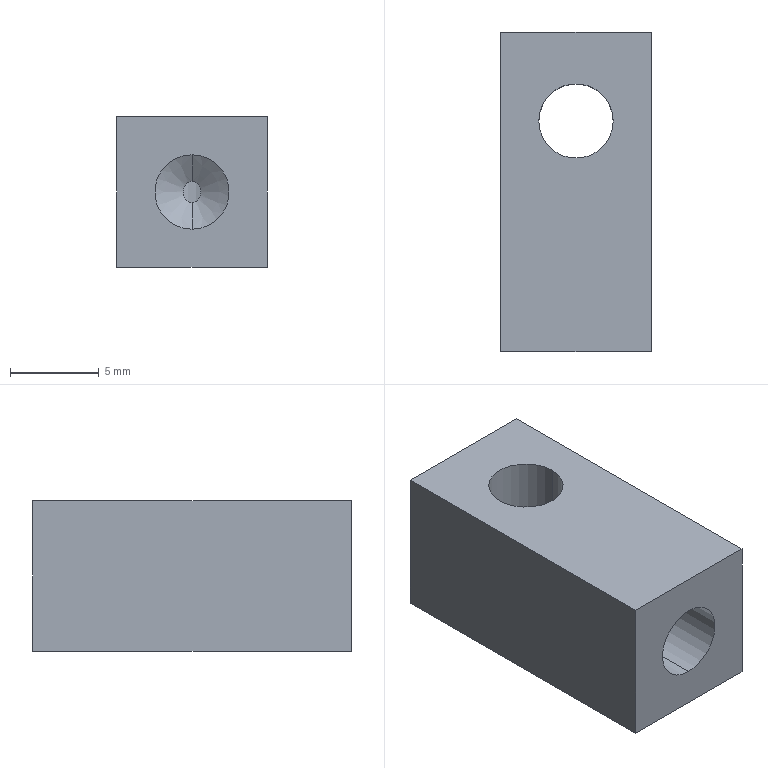Part | STEP file | Stopper | 1 solid | 12 faces | box 8.5 x 18 x 8.5 mm | volume 1038 mm3 | plane 6 | cylinder 4 | cone 2 | commonest cylinder face diameters 4.2 x4
STEP:
#1=CARTESIAN_POINT('',(0.,0.,0.));
#2=DIRECTION('',(0.,0.,1.));
#3=DIRECTION('',(1.,0.,0.));
#4=AXIS2_PLACEMENT_3D('',#1,#2,#3);
#5=CARTESIAN_POINT('',(4.25,10.,2.15));
#6=VERTEX_POINT('',#5);
#7=CARTESIAN_POINT('',(4.25,0.,2.15));
#8=VERTEX_POINT('',#7);
#9=CARTESIAN_POINT('',(4.25,0.,2.15));
#10=DIRECTION('',(0.,-1.,0.));
#11=VECTOR('',#10,1.);
#12=LINE('',#9,#11);
#13=CARTESIAN_POINT('',(4.25,0.,4.25));
#14=DIRECTION('',(0.,-1.,0.));
#15=DIRECTION('',(0.,0.,-1.));
#16=AXIS2_PLACEMENT_3D('',#13,#14,#15);
#17=CYLINDRICAL_SURFACE('',#16,2.1);
#18=CARTESIAN_POINT('',(6.283,0.));
#19=DIRECTION('',(0.,1.));
#20=VECTOR('',#19,1.);
#21=LINE('',#18,#20);
#22=(GEOMETRIC_REPRESENTATION_CONTEXT(2)PARAMETRIC_REPRESENTATION_CONTEXT()REPRESENTATION_CONTEXT('',''));
#23=DEFINITIONAL_REPRESENTATION('',(#21),#22);
#24=PCURVE('',#17,#23);
#25=CARTESIAN_POINT('',(4.25,0.,4.25));
#26=DIRECTION('',(0.,-1.,0.));
#27=DIRECTION('',(0.,0.,-1.));
#28=AXIS2_PLACEMENT_3D('',#25,#26,#27);
#29=CYLINDRICAL_SURFACE('',#28,2.1);
#30=CARTESIAN_POINT('',(0.,0.));
#31=DIRECTION('',(0.,1.));
#32=VECTOR('',#31,1.);
#33=LINE('',#30,#32);
#34=(GEOMETRIC_REPRESENTATION_CONTEXT(2)PARAMETRIC_REPRESENTATION_CONTEXT()REPRESENTATION_CONTEXT('',''));
#35=DEFINITIONAL_REPRESENTATION('',(#33),#34);
#36=PCURVE('',#29,#35);
#37=SURFACE_CURVE('',#12,(#24,#36),.PCURVE_S1.);
#38=EDGE_CURVE('',#6,#8,#37,.T.);
#39=ORIENTED_EDGE('',*,*,#38,.T.);
#40=CARTESIAN_POINT('',(4.25,0.,6.35));
#41=VERTEX_POINT('',#40);
#42=CARTESIAN_POINT('',(4.25,0.,4.25));
#43=DIRECTION('',(0.,-1.,0.));
#44=DIRECTION('',(0.,0.,-1.));
#45=AXIS2_PLACEMENT_3D('',#42,#43,#44);
#46=CIRCLE('',#45,2.1);
#47=CARTESIAN_POINT('',(0.,0.));
#48=DIRECTION('',(1.,0.));
#49=VECTOR('',#48,1.);
#50=LINE('',#47,#49);
#51=(GEOMETRIC_REPRESENTATION_CONTEXT(2)PARAMETRIC_REPRESENTATION_CONTEXT()REPRESENTATION_CONTEXT('',''));
#52=DEFINITIONAL_REPRESENTATION('',(#50),#51);
#53=PCURVE('',#17,#52);
#54=CARTESIAN_POINT('',(0.,0.,8.5));
#55=DIRECTION('',(0.,1.,0.));
#56=DIRECTION('',(0.,0.,1.));
#57=AXIS2_PLACEMENT_3D('',#54,#55,#56);
#58=PLANE('',#57);
#59=CARTESIAN_POINT('',(-6.35,4.25));
#60=CARTESIAN_POINT('',(-6.35,7.887));
#61=CARTESIAN_POINT('',(-3.2,6.069));
#62=CARTESIAN_POINT('',(-0.05,4.25));
#63=CARTESIAN_POINT('',(-3.2,2.431));
#64=CARTESIAN_POINT('',(-6.35,0.6127));
#65=CARTESIAN_POINT('',(-6.35,4.25));
#66=(BOUNDED_CURVE()B_SPLINE_CURVE(2,(#59,#60,#61,#62,#63,#64,#65),.UNSPECIFIED.,.T.,.F.)B_SPLINE_CURVE_WITH_KNOTS((1,2,2,2,2,1),(-2.094,0.,2.094,4.189,6.283,8.378),.UNSPECIFIED.)CURVE()GEOMETRIC_REPRESENTATION_ITEM()RATIONAL_B_SPLINE_CURVE((1.,0.5,1.,0.5,1.,0.5,1.))REPRESENTATION_ITEM(''));
#67=(GEOMETRIC_REPRESENTATION_CONTEXT(2)PARAMETRIC_REPRESENTATION_CONTEXT()REPRESENTATION_CONTEXT('',''));
#68=DEFINITIONAL_REPRESENTATION('',(#66),#67);
#69=PCURVE('',#58,#68);
#70=SURFACE_CURVE('',#46,(#53,#69),.PCURVE_S1.);
#71=EDGE_CURVE('',#41,#8,#70,.T.);
#72=ORIENTED_EDGE('',*,*,#71,.F.);
#73=CARTESIAN_POINT('',(4.25,10.,6.35));
#74=VERTEX_POINT('',#73);
#75=CARTESIAN_POINT('',(4.25,0.,6.35));
#76=DIRECTION('',(0.,-1.,0.));
#77=VECTOR('',#76,1.);
#78=LINE('',#75,#77);
#79=CARTESIAN_POINT('',(3.142,0.));
#80=DIRECTION('',(0.,1.));
#81=VECTOR('',#80,1.);
#82=LINE('',#79,#81);
#83=(GEOMETRIC_REPRESENTATION_CONTEXT(2)PARAMETRIC_REPRESENTATION_CONTEXT()REPRESENTATION_CONTEXT('',''));
#84=DEFINITIONAL_REPRESENTATION('',(#82),#83);
#85=PCURVE('',#17,#84);
#86=CARTESIAN_POINT('',(3.142,0.));
#87=DIRECTION('',(0.,1.));
#88=VECTOR('',#87,1.);
#89=LINE('',#86,#88);
#90=(GEOMETRIC_REPRESENTATION_CONTEXT(2)PARAMETRIC_REPRESENTATION_CONTEXT()REPRESENTATION_CONTEXT('',''));
#91=DEFINITIONAL_REPRESENTATION('',(#89),#90);
#92=PCURVE('',#29,#91);
#93=SURFACE_CURVE('',#78,(#85,#92),.PCURVE_S1.);
#94=EDGE_CURVE('',#74,#41,#93,.T.);
#95=ORIENTED_EDGE('',*,*,#94,.F.);
#96=CARTESIAN_POINT('',(4.25,10.,4.25));
#97=DIRECTION('',(0.,-1.,0.));
#98=DIRECTION('',(0.,0.,-1.));
#99=AXIS2_PLACEMENT_3D('',#96,#97,#98);
#100=CIRCLE('',#99,2.1);
#101=CARTESIAN_POINT('',(0.,-10.));
#102=DIRECTION('',(1.,0.));
#103=VECTOR('',#102,1.);
#104=LINE('',#101,#103);
#105=(GEOMETRIC_REPRESENTATION_CONTEXT(2)PARAMETRIC_REPRESENTATION_CONTEXT()REPRESENTATION_CONTEXT('',''));
#106=DEFINITIONAL_REPRESENTATION('',(#104),#105);
#107=PCURVE('',#17,#106);
#108=CARTESIAN_POINT('',(4.25,10.,4.25));
#109=DIRECTION('',(0.,-1.,0.));
#110=DIRECTION('',(0.,0.,-1.));
#111=AXIS2_PLACEMENT_3D('',#108,#109,#110);
#112=CONICAL_SURFACE('',#111,2.1,1.03);
#113=CARTESIAN_POINT('',(0.,0.));
#114=DIRECTION('',(1.,0.));
#115=VECTOR('',#114,1.);
#116=LINE('',#113,#115);
#117=(GEOMETRIC_REPRESENTATION_CONTEXT(2)PARAMETRIC_REPRESENTATION_CONTEXT()REPRESENTATION_CONTEXT('',''));
#118=DEFINITIONAL_REPRESENTATION('',(#116),#117);
#119=PCURVE('',#112,#118);
#120=SURFACE_CURVE('',#100,(#107,#119),.PCURVE_S1.);
#121=EDGE_CURVE('',#74,#6,#120,.T.);
#122=ORIENTED_EDGE('',*,*,#121,.T.);
#123=EDGE_LOOP('',(#39,#72,#95,#122));
#124=FACE_BOUND('',#123,.F.);
#125=ADVANCED_FACE('',(#124),#17,.F.);
#126=CARTESIAN_POINT('',(4.25,10.9,3.648));
#127=VERTEX_POINT('',#126);
#128=CARTESIAN_POINT('',(4.25,10.,2.15));
#129=DIRECTION('',(0.,-0.515,-0.8572));
#130=VECTOR('',#129,1.);
#131=LINE('',#128,#130);
#132=CARTESIAN_POINT('',(6.283,0.));
#133=DIRECTION('',(0.,1.));
#134=VECTOR('',#133,1.);
#135=LINE('',#132,#134);
#136=(GEOMETRIC_REPRESENTATION_CONTEXT(2)PARAMETRIC_REPRESENTATION_CONTEXT()REPRESENTATION_CONTEXT('',''));
#137=DEFINITIONAL_REPRESENTATION('',(#135),#136);
#138=PCURVE('',#112,#137);
#139=CARTESIAN_POINT('',(4.25,10.,4.25));
#140=DIRECTION('',(0.,-1.,0.));
#141=DIRECTION('',(0.,0.,-1.));
#142=AXIS2_PLACEMENT_3D('',#139,#140,#141);
#143=CONICAL_SURFACE('',#142,2.1,1.03);
#144=CARTESIAN_POINT('',(0.,0.));
#145=DIRECTION('',(0.,1.));
#146=VECTOR('',#145,1.);
#147=LINE('',#144,#146);
#148=(GEOMETRIC_REPRESENTATION_CONTEXT(2)PARAMETRIC_REPRESENTATION_CONTEXT()REPRESENTATION_CONTEXT('',''));
#149=DEFINITIONAL_REPRESENTATION('',(#147),#148);
#150=PCURVE('',#143,#149);
#151=SURFACE_CURVE('',#131,(#138,#150),.PCURVE_S1.);
#152=EDGE_CURVE('',#127,#6,#151,.T.);
#153=ORIENTED_EDGE('',*,*,#152,.T.);
#154=ORIENTED_EDGE('',*,*,#121,.F.);
#155=CARTESIAN_POINT('',(4.25,10.9,4.852));
#156=VERTEX_POINT('',#155);
#157=CARTESIAN_POINT('',(4.25,10.,6.35));
#158=DIRECTION('',(0.,-0.515,0.8572));
#159=VECTOR('',#158,1.);
#160=LINE('',#157,#159);
#161=CARTESIAN_POINT('',(3.142,0.));
#162=DIRECTION('',(0.,1.));
#163=VECTOR('',#162,1.);
#164=LINE('',#161,#163);
#165=(GEOMETRIC_REPRESENTATION_CONTEXT(2)PARAMETRIC_REPRESENTATION_CONTEXT()REPRESENTATION_CONTEXT('',''));
#166=DEFINITIONAL_REPRESENTATION('',(#164),#165);
#167=PCURVE('',#112,#166);
#168=CARTESIAN_POINT('',(3.142,0.));
#169=DIRECTION('',(0.,1.));
#170=VECTOR('',#169,1.);
#171=LINE('',#168,#170);
#172=(GEOMETRIC_REPRESENTATION_CONTEXT(2)PARAMETRIC_REPRESENTATION_CONTEXT()REPRESENTATION_CONTEXT('',''));
#173=DEFINITIONAL_REPRESENTATION('',(#171),#172);
#174=PCURVE('',#143,#173);
#175=SURFACE_CURVE('',#160,(#167,#174),.PCURVE_S1.);
#176=EDGE_CURVE('',#156,#74,#175,.T.);
#177=ORIENTED_EDGE('',*,*,#176,.F.);
#178=CARTESIAN_POINT('',(4.25,10.9,4.852));
#179=CARTESIAN_POINT('',(4.178,10.9,4.852));
#180=CARTESIAN_POINT('',(4.105,10.904,4.832));
#181=CARTESIAN_POINT('',(3.979,10.917,4.761));
#182=CARTESIAN_POINT('',(3.924,10.925,4.712));
#183=CARTESIAN_POINT('',(3.794,10.948,4.54));
#184=CARTESIAN_POINT('',(3.749,10.961,4.394));
#185=CARTESIAN_POINT('',(3.749,10.961,4.104));
#186=CARTESIAN_POINT('',(3.794,10.948,3.959));
#187=CARTESIAN_POINT('',(3.926,10.925,3.787));
#188=CARTESIAN_POINT('',(3.98,10.916,3.738));
#189=CARTESIAN_POINT('',(4.106,10.904,3.668));
#190=CARTESIAN_POINT('',(4.178,10.9,3.648));
#191=CARTESIAN_POINT('',(4.25,10.9,3.648));
#192=B_SPLINE_CURVE_WITH_KNOTS('',3,(#178,#179,#180,#181,#182,#183,#184,#185,#186,#187,#188,#189,#190,#191),.UNSPECIFIED.,.F.,.F.,(4,2,2,2,2,2,4),(0.002401,0.002617,0.002832,0.003263,0.003694,0.003909,0.004125),.UNSPECIFIED.);
#193=CARTESIAN_POINT('',(3.142,-0.9));
#194=CARTESIAN_POINT('',(3.163,-0.9));
#195=CARTESIAN_POINT('',(3.207,-0.9003));
#196=CARTESIAN_POINT('',(3.273,-0.9014));
#197=CARTESIAN_POINT('',(3.339,-0.9033));
#198=CARTESIAN_POINT('',(3.405,-0.9057));
#199=CARTESIAN_POINT('',(3.472,-0.9086));
#200=CARTESIAN_POINT('',(3.539,-0.912));
#201=CARTESIAN_POINT('',(3.606,-0.9159));
#202=CARTESIAN_POINT('',(3.674,-0.9199));
#203=CARTESIAN_POINT('',(3.742,-0.9242));
#204=CARTESIAN_POINT('',(3.812,-0.9285));
#205=CARTESIAN_POINT('',(3.882,-0.9328));
#206=CARTESIAN_POINT('',(3.953,-0.937));
#207=CARTESIAN_POINT('',(4.025,-0.941));
#208=CARTESIAN_POINT('',(4.098,-0.9448));
#209=CARTESIAN_POINT('',(4.172,-0.9483));
#210=CARTESIAN_POINT('',(4.247,-0.9514));
#211=CARTESIAN_POINT('',(4.324,-0.9542));
#212=CARTESIAN_POINT('',(4.401,-0.9565));
#213=CARTESIAN_POINT('',(4.479,-0.9584));
#214=CARTESIAN_POINT('',(4.557,-0.9597));
#215=CARTESIAN_POINT('',(4.636,-0.9605));
#216=CARTESIAN_POINT('',(4.714,-0.9608));
#217=CARTESIAN_POINT('',(4.793,-0.9605));
#218=CARTESIAN_POINT('',(4.872,-0.9596));
#219=CARTESIAN_POINT('',(4.95,-0.9583));
#220=CARTESIAN_POINT('',(5.028,-0.9564));
#221=CARTESIAN_POINT('',(5.105,-0.9541));
#222=CARTESIAN_POINT('',(5.181,-0.9513));
#223=CARTESIAN_POINT('',(5.256,-0.9481));
#224=CARTESIAN_POINT('',(5.33,-0.9446));
#225=CARTESIAN_POINT('',(5.403,-0.9408));
#226=CARTESIAN_POINT('',(5.475,-0.9368));
#227=CARTESIAN_POINT('',(5.546,-0.9326));
#228=CARTESIAN_POINT('',(5.617,-0.9283));
#229=CARTESIAN_POINT('',(5.686,-0.924));
#230=CARTESIAN_POINT('',(5.754,-0.9197));
#231=CARTESIAN_POINT('',(5.821,-0.9157));
#232=CARTESIAN_POINT('',(5.888,-0.9119));
#233=CARTESIAN_POINT('',(5.954,-0.9085));
#234=CARTESIAN_POINT('',(6.021,-0.9056));
#235=CARTESIAN_POINT('',(6.086,-0.9032));
#236=CARTESIAN_POINT('',(6.152,-0.9014));
#237=CARTESIAN_POINT('',(6.218,-0.9003));
#238=CARTESIAN_POINT('',(6.261,-0.9));
#239=CARTESIAN_POINT('',(6.283,-0.9));
#240=B_SPLINE_CURVE_WITH_KNOTS('',3,(#193,#194,#195,#196,#197,#198,#199,#200,#201,#202,#203,#204,#205,#206,#207,#208,#209,#210,#211,#212,#213,#214,#215,#216,#217,#218,#219,#220,#221,#222,#223,#224,#225,#226,#227,#228,#229,#230,#231,#232,#233,#234,#235,#236,#237,#238,#239),.UNSPECIFIED.,.F.,.F.,(4,1,1,1,1,1,1,1,1,1,1,1,1,1,1,1,1,1,1,1,1,1,1,1,1,1,1,1,1,1,1,1,1,1,1,1,1,1,1,1,1,1,1,1,4),(0.002401,0.00244,0.002479,0.002519,0.002558,0.002597,0.002636,0.002675,0.002714,0.002754,0.002793,0.002832,0.002871,0.00291,0.00295,0.002989,0.003028,0.003067,0.003106,0.003145,0.003185,0.003224,0.003263,0.003302,0.003341,0.00338,0.00342,0.003459,0.003498,0.003537,0.003576,0.003616,0.003655,0.003694,0.003733,0.003772,0.003811,0.003851,0.00389,0.003929,0.003968,0.004007,0.004046,0.004086,0.004125),.QUASI_UNIFORM_KNOTS.);
#241=(GEOMETRIC_REPRESENTATION_CONTEXT(2)PARAMETRIC_REPRESENTATION_CONTEXT()REPRESENTATION_CONTEXT('',''));
#242=DEFINITIONAL_REPRESENTATION('',(#240),#241);
#243=PCURVE('',#112,#242);
#244=CARTESIAN_POINT('',(4.25,13.,8.5));
#245=DIRECTION('',(0.,0.,1.));
#246=DIRECTION('',(1.,0.,0.));
#247=AXIS2_PLACEMENT_3D('',#244,#245,#246);
#248=CYLINDRICAL_SURFACE('',#247,2.1);
#249=CARTESIAN_POINT('',(4.712,-3.648));
#250=CARTESIAN_POINT('',(4.706,-3.648));
#251=CARTESIAN_POINT('',(4.694,-3.649));
#252=CARTESIAN_POINT('',(4.675,-3.655));
#253=CARTESIAN_POINT('',(4.657,-3.664));
#254=CARTESIAN_POINT('',(4.639,-3.677));
#255=CARTESIAN_POINT('',(4.621,-3.694));
#256=CARTESIAN_POINT('',(4.605,-3.713));
#257=CARTESIAN_POINT('',(4.589,-3.735));
#258=CARTESIAN_POINT('',(4.574,-3.759));
#259=CARTESIAN_POINT('',(4.56,-3.786));
#260=CARTESIAN_POINT('',(4.547,-3.815));
#261=CARTESIAN_POINT('',(4.535,-3.845));
#262=CARTESIAN_POINT('',(4.524,-3.877));
#263=CARTESIAN_POINT('',(4.514,-3.911));
#264=CARTESIAN_POINT('',(4.505,-3.946));
#265=CARTESIAN_POINT('',(4.497,-3.981));
#266=CARTESIAN_POINT('',(4.491,-4.018));
#267=CARTESIAN_POINT('',(4.485,-4.056));
#268=CARTESIAN_POINT('',(4.48,-4.094));
#269=CARTESIAN_POINT('',(4.476,-4.133));
#270=CARTESIAN_POINT('',(4.473,-4.172));
#271=CARTESIAN_POINT('',(4.472,-4.212));
#272=CARTESIAN_POINT('',(4.471,-4.251));
#273=CARTESIAN_POINT('',(4.472,-4.29));
#274=CARTESIAN_POINT('',(4.473,-4.33));
#275=CARTESIAN_POINT('',(4.476,-4.369));
#276=CARTESIAN_POINT('',(4.48,-4.408));
#277=CARTESIAN_POINT('',(4.485,-4.446));
#278=CARTESIAN_POINT('',(4.491,-4.483));
#279=CARTESIAN_POINT('',(4.498,-4.52));
#280=CARTESIAN_POINT('',(4.506,-4.556));
#281=CARTESIAN_POINT('',(4.515,-4.591));
#282=CARTESIAN_POINT('',(4.525,-4.624));
#283=CARTESIAN_POINT('',(4.536,-4.656));
#284=CARTESIAN_POINT('',(4.548,-4.687));
#285=CARTESIAN_POINT('',(4.561,-4.715));
#286=CARTESIAN_POINT('',(4.575,-4.742));
#287=CARTESIAN_POINT('',(4.59,-4.766));
#288=CARTESIAN_POINT('',(4.605,-4.788));
#289=CARTESIAN_POINT('',(4.622,-4.807));
#290=CARTESIAN_POINT('',(4.639,-4.823));
#291=CARTESIAN_POINT('',(4.657,-4.836));
#292=CARTESIAN_POINT('',(4.675,-4.845));
#293=CARTESIAN_POINT('',(4.694,-4.851));
#294=CARTESIAN_POINT('',(4.706,-4.852));
#295=CARTESIAN_POINT('',(4.712,-4.852));
#296=B_SPLINE_CURVE_WITH_KNOTS('',3,(#249,#250,#251,#252,#253,#254,#255,#256,#257,#258,#259,#260,#261,#262,#263,#264,#265,#266,#267,#268,#269,#270,#271,#272,#273,#274,#275,#276,#277,#278,#279,#280,#281,#282,#283,#284,#285,#286,#287,#288,#289,#290,#291,#292,#293,#294,#295),.UNSPECIFIED.,.F.,.F.,(4,1,1,1,1,1,1,1,1,1,1,1,1,1,1,1,1,1,1,1,1,1,1,1,1,1,1,1,1,1,1,1,1,1,1,1,1,1,1,1,1,1,1,1,4),(0.002401,0.00244,0.002479,0.002519,0.002558,0.002597,0.002636,0.002675,0.002714,0.002754,0.002793,0.002832,0.002871,0.00291,0.00295,0.002989,0.003028,0.003067,0.003106,0.003145,0.003185,0.003224,0.003263,0.003302,0.003341,0.00338,0.00342,0.003459,0.003498,0.003537,0.003576,0.003616,0.003655,0.003694,0.003733,0.003772,0.003811,0.003851,0.00389,0.003929,0.003968,0.004007,0.004046,0.004086,0.004125),.QUASI_UNIFORM_KNOTS.);
#297=(GEOMETRIC_REPRESENTATION_CONTEXT(2)PARAMETRIC_REPRESENTATION_CONTEXT()REPRESENTATION_CONTEXT('',''));
#298=DEFINITIONAL_REPRESENTATION('',(#296),#297);
#299=PCURVE('',#248,#298);
#300=SURFACE_CURVE('',#192,(#243,#299),.PCURVE_S1.);
#301=EDGE_CURVE('',#156,#127,#300,.T.);
#302=ORIENTED_EDGE('',*,*,#301,.T.);
#303=EDGE_LOOP('',(#153,#154,#177,#302));
#304=FACE_BOUND('',#303,.F.);
#305=ADVANCED_FACE('',(#304),#112,.F.);
#306=ORIENTED_EDGE('',*,*,#301,.F.);
#307=CARTESIAN_POINT('',(4.25,10.9,3.648));
#308=CARTESIAN_POINT('',(4.322,10.9,3.648));
#309=CARTESIAN_POINT('',(4.395,10.904,3.668));
#310=CARTESIAN_POINT('',(4.521,10.917,3.738));
#311=CARTESIAN_POINT('',(4.576,10.925,3.788));
#312=CARTESIAN_POINT('',(4.707,10.948,3.961));
#313=CARTESIAN_POINT('',(4.751,10.961,4.105));
#314=CARTESIAN_POINT('',(4.751,10.961,4.397));
#315=CARTESIAN_POINT('',(4.706,10.948,4.54));
#316=CARTESIAN_POINT('',(4.576,10.925,4.712));
#317=CARTESIAN_POINT('',(4.521,10.917,4.762));
#318=CARTESIAN_POINT('',(4.394,10.904,4.832));
#319=CARTESIAN_POINT('',(4.322,10.9,4.852));
#320=CARTESIAN_POINT('',(4.25,10.9,4.852));
#321=B_SPLINE_CURVE_WITH_KNOTS('',3,(#307,#308,#309,#310,#311,#312,#313,#314,#315,#316,#317,#318,#319,#320),.UNSPECIFIED.,.F.,.F.,(4,2,2,2,2,2,4),(0.000676,0.0008917,0.001107,0.001539,0.00197,0.002185,0.002401),.UNSPECIFIED.);
#322=CARTESIAN_POINT('',(4.712,-4.852));
#323=CARTESIAN_POINT('',(4.719,-4.852));
#324=CARTESIAN_POINT('',(4.731,-4.851));
#325=CARTESIAN_POINT('',(4.75,-4.845));
#326=CARTESIAN_POINT('',(4.768,-4.835));
#327=CARTESIAN_POINT('',(4.786,-4.823));
#328=CARTESIAN_POINT('',(4.803,-4.806));
#329=CARTESIAN_POINT('',(4.82,-4.787));
#330=CARTESIAN_POINT('',(4.836,-4.765));
#331=CARTESIAN_POINT('',(4.85,-4.741));
#332=CARTESIAN_POINT('',(4.864,-4.714));
#333=CARTESIAN_POINT('',(4.877,-4.685));
#334=CARTESIAN_POINT('',(4.889,-4.655));
#335=CARTESIAN_POINT('',(4.9,-4.623));
#336=CARTESIAN_POINT('',(4.91,-4.589));
#337=CARTESIAN_POINT('',(4.919,-4.555));
#338=CARTESIAN_POINT('',(4.927,-4.519));
#339=CARTESIAN_POINT('',(4.934,-4.482));
#340=CARTESIAN_POINT('',(4.94,-4.445));
#341=CARTESIAN_POINT('',(4.945,-4.407));
#342=CARTESIAN_POINT('',(4.949,-4.368));
#343=CARTESIAN_POINT('',(4.951,-4.329));
#344=CARTESIAN_POINT('',(4.953,-4.289));
#345=CARTESIAN_POINT('',(4.954,-4.249));
#346=CARTESIAN_POINT('',(4.953,-4.21));
#347=CARTESIAN_POINT('',(4.951,-4.17));
#348=CARTESIAN_POINT('',(4.949,-4.131));
#349=CARTESIAN_POINT('',(4.945,-4.092));
#350=CARTESIAN_POINT('',(4.94,-4.054));
#351=CARTESIAN_POINT('',(4.934,-4.017));
#352=CARTESIAN_POINT('',(4.927,-3.98));
#353=CARTESIAN_POINT('',(4.919,-3.945));
#354=CARTESIAN_POINT('',(4.91,-3.91));
#355=CARTESIAN_POINT('',(4.9,-3.877));
#356=CARTESIAN_POINT('',(4.889,-3.845));
#357=CARTESIAN_POINT('',(4.877,-3.815));
#358=CARTESIAN_POINT('',(4.864,-3.786));
#359=CARTESIAN_POINT('',(4.85,-3.759));
#360=CARTESIAN_POINT('',(4.836,-3.735));
#361=CARTESIAN_POINT('',(4.82,-3.713));
#362=CARTESIAN_POINT('',(4.803,-3.693));
#363=CARTESIAN_POINT('',(4.786,-3.677));
#364=CARTESIAN_POINT('',(4.768,-3.664));
#365=CARTESIAN_POINT('',(4.75,-3.655));
#366=CARTESIAN_POINT('',(4.731,-3.649));
#367=CARTESIAN_POINT('',(4.719,-3.648));
#368=CARTESIAN_POINT('',(4.712,-3.648));
#369=B_SPLINE_CURVE_WITH_KNOTS('',3,(#322,#323,#324,#325,#326,#327,#328,#329,#330,#331,#332,#333,#334,#335,#336,#337,#338,#339,#340,#341,#342,#343,#344,#345,#346,#347,#348,#349,#350,#351,#352,#353,#354,#355,#356,#357,#358,#359,#360,#361,#362,#363,#364,#365,#366,#367,#368),.UNSPECIFIED.,.F.,.F.,(4,1,1,1,1,1,1,1,1,1,1,1,1,1,1,1,1,1,1,1,1,1,1,1,1,1,1,1,1,1,1,1,1,1,1,1,1,1,1,1,1,1,1,1,4),(0.000676,0.0007152,0.0007544,0.0007937,0.0008329,0.0008721,0.0009113,0.0009505,0.0009897,0.001029,0.001068,0.001107,0.001146,0.001186,0.001225,0.001264,0.001303,0.001343,0.001382,0.001421,0.00146,0.001499,0.001539,0.001578,0.001617,0.001656,0.001695,0.001735,0.001774,0.001813,0.001852,0.001891,0.001931,0.00197,0.002009,0.002048,0.002087,0.002127,0.002166,0.002205,0.002244,0.002283,0.002323,0.002362,0.002401),.QUASI_UNIFORM_KNOTS.);
#370=(GEOMETRIC_REPRESENTATION_CONTEXT(2)PARAMETRIC_REPRESENTATION_CONTEXT()REPRESENTATION_CONTEXT('',''));
#371=DEFINITIONAL_REPRESENTATION('',(#369),#370);
#372=PCURVE('',#248,#371);
#373=CARTESIAN_POINT('',(0.,-0.9));
#374=CARTESIAN_POINT('',(0.02187,-0.9));
#375=CARTESIAN_POINT('',(0.06565,-0.9003));
#376=CARTESIAN_POINT('',(0.1315,-0.9014));
#377=CARTESIAN_POINT('',(0.1975,-0.9033));
#378=CARTESIAN_POINT('',(0.2638,-0.9057));
#379=CARTESIAN_POINT('',(0.3303,-0.9086));
#380=CARTESIAN_POINT('',(0.3969,-0.912));
#381=CARTESIAN_POINT('',(0.4639,-0.9158));
#382=CARTESIAN_POINT('',(0.5316,-0.9199));
#383=CARTESIAN_POINT('',(0.6002,-0.9241));
#384=CARTESIAN_POINT('',(0.6696,-0.9284));
#385=CARTESIAN_POINT('',(0.7399,-0.9327));
#386=CARTESIAN_POINT('',(0.811,-0.9369));
#387=CARTESIAN_POINT('',(0.883,-0.9409));
#388=CARTESIAN_POINT('',(0.956,-0.9447));
#389=CARTESIAN_POINT('',(1.03,-0.9482));
#390=CARTESIAN_POINT('',(1.105,-0.9513));
#391=CARTESIAN_POINT('',(1.181,-0.9541));
#392=CARTESIAN_POINT('',(1.258,-0.9564));
#393=CARTESIAN_POINT('',(1.336,-0.9583));
#394=CARTESIAN_POINT('',(1.414,-0.9597));
#395=CARTESIAN_POINT('',(1.493,-0.9605));
#396=CARTESIAN_POINT('',(1.572,-0.9608));
#397=CARTESIAN_POINT('',(1.652,-0.9605));
#398=CARTESIAN_POINT('',(1.73,-0.9596));
#399=CARTESIAN_POINT('',(1.809,-0.9582));
#400=CARTESIAN_POINT('',(1.886,-0.9563));
#401=CARTESIAN_POINT('',(1.963,-0.954));
#402=CARTESIAN_POINT('',(2.038,-0.9512));
#403=CARTESIAN_POINT('',(2.113,-0.9481));
#404=CARTESIAN_POINT('',(2.187,-0.9446));
#405=CARTESIAN_POINT('',(2.259,-0.9409));
#406=CARTESIAN_POINT('',(2.331,-0.9369));
#407=CARTESIAN_POINT('',(2.402,-0.9327));
#408=CARTESIAN_POINT('',(2.472,-0.9284));
#409=CARTESIAN_POINT('',(2.542,-0.9241));
#410=CARTESIAN_POINT('',(2.61,-0.9199));
#411=CARTESIAN_POINT('',(2.678,-0.9158));
#412=CARTESIAN_POINT('',(2.745,-0.912));
#413=CARTESIAN_POINT('',(2.812,-0.9086));
#414=CARTESIAN_POINT('',(2.879,-0.9056));
#415=CARTESIAN_POINT('',(2.945,-0.9032));
#416=CARTESIAN_POINT('',(3.011,-0.9014));
#417=CARTESIAN_POINT('',(3.076,-0.9003));
#418=CARTESIAN_POINT('',(3.12,-0.9));
#419=CARTESIAN_POINT('',(3.142,-0.9));
#420=B_SPLINE_CURVE_WITH_KNOTS('',3,(#373,#374,#375,#376,#377,#378,#379,#380,#381,#382,#383,#384,#385,#386,#387,#388,#389,#390,#391,#392,#393,#394,#395,#396,#397,#398,#399,#400,#401,#402,#403,#404,#405,#406,#407,#408,#409,#410,#411,#412,#413,#414,#415,#416,#417,#418,#419),.UNSPECIFIED.,.F.,.F.,(4,1,1,1,1,1,1,1,1,1,1,1,1,1,1,1,1,1,1,1,1,1,1,1,1,1,1,1,1,1,1,1,1,1,1,1,1,1,1,1,1,1,1,1,4),(0.000676,0.0007152,0.0007544,0.0007937,0.0008329,0.0008721,0.0009113,0.0009505,0.0009897,0.001029,0.001068,0.001107,0.001146,0.001186,0.001225,0.001264,0.001303,0.001343,0.001382,0.001421,0.00146,0.001499,0.001539,0.001578,0.001617,0.001656,0.001695,0.001735,0.001774,0.001813,0.001852,0.001891,0.001931,0.00197,0.002009,0.002048,0.002087,0.002127,0.002166,0.002205,0.002244,0.002283,0.002323,0.002362,0.002401),.QUASI_UNIFORM_KNOTS.);
#421=(GEOMETRIC_REPRESENTATION_CONTEXT(2)PARAMETRIC_REPRESENTATION_CONTEXT()REPRESENTATION_CONTEXT('',''));
#422=DEFINITIONAL_REPRESENTATION('',(#420),#421);
#423=PCURVE('',#143,#422);
#424=SURFACE_CURVE('',#321,(#372,#423),.PCURVE_S1.);
#425=EDGE_CURVE('',#127,#156,#424,.T.);
#426=ORIENTED_EDGE('',*,*,#425,.F.);
#427=EDGE_LOOP('',(#306,#426));
#428=FACE_BOUND('',#427,.F.);
#429=CARTESIAN_POINT('',(6.35,13.,0.));
#430=VERTEX_POINT('',#429);
#431=CARTESIAN_POINT('',(6.35,13.,8.5));
#432=VERTEX_POINT('',#431);
#433=CARTESIAN_POINT('',(6.35,13.,8.5));
#434=DIRECTION('',(0.,0.,1.));
#435=VECTOR('',#434,1.);
#436=LINE('',#433,#435);
#437=CARTESIAN_POINT('',(6.283,0.));
#438=DIRECTION('',(0.,1.));
#439=VECTOR('',#438,1.);
#440=LINE('',#437,#439);
#441=(GEOMETRIC_REPRESENTATION_CONTEXT(2)PARAMETRIC_REPRESENTATION_CONTEXT()REPRESENTATION_CONTEXT('',''));
#442=DEFINITIONAL_REPRESENTATION('',(#440),#441);
#443=PCURVE('',#248,#442);
#444=CARTESIAN_POINT('',(4.25,13.,8.5));
#445=DIRECTION('',(0.,0.,1.));
#446=DIRECTION('',(1.,0.,0.));
#447=AXIS2_PLACEMENT_3D('',#444,#445,#446);
#448=CYLINDRICAL_SURFACE('',#447,2.1);
#449=CARTESIAN_POINT('',(0.,0.));
#450=DIRECTION('',(0.,1.));
#451=VECTOR('',#450,1.);
#452=LINE('',#449,#451);
#453=(GEOMETRIC_REPRESENTATION_CONTEXT(2)PARAMETRIC_REPRESENTATION_CONTEXT()REPRESENTATION_CONTEXT('',''));
#454=DEFINITIONAL_REPRESENTATION('',(#452),#453);
#455=PCURVE('',#448,#454);
#456=SURFACE_CURVE('',#436,(#443,#455),.PCURVE_S1.);
#457=EDGE_CURVE('',#430,#432,#456,.T.);
#458=ORIENTED_EDGE('',*,*,#457,.T.);
#459=CARTESIAN_POINT('',(2.15,13.,8.5));
#460=VERTEX_POINT('',#459);
#461=CARTESIAN_POINT('',(4.25,13.,8.5));
#462=DIRECTION('',(0.,0.,1.));
#463=DIRECTION('',(1.,0.,0.));
#464=AXIS2_PLACEMENT_3D('',#461,#462,#463);
#465=CIRCLE('',#464,2.1);
#466=CARTESIAN_POINT('',(0.,0.));
#467=DIRECTION('',(1.,0.));
#468=VECTOR('',#467,1.);
#469=LINE('',#466,#468);
#470=(GEOMETRIC_REPRESENTATION_CONTEXT(2)PARAMETRIC_REPRESENTATION_CONTEXT()REPRESENTATION_CONTEXT('',''));
#471=DEFINITIONAL_REPRESENTATION('',(#469),#470);
#472=PCURVE('',#248,#471);
#473=CARTESIAN_POINT('',(0.,18.,8.5));
#474=DIRECTION('',(0.,0.,-1.));
#475=DIRECTION('',(-1.,0.,0.));
#476=AXIS2_PLACEMENT_3D('',#473,#474,#475);
#477=PLANE('',#476);
#478=CARTESIAN_POINT('',(-6.35,-5.));
#479=CARTESIAN_POINT('',(-6.35,-1.363));
#480=CARTESIAN_POINT('',(-3.2,-3.181));
#481=CARTESIAN_POINT('',(-0.05,-5.));
#482=CARTESIAN_POINT('',(-3.2,-6.819));
#483=CARTESIAN_POINT('',(-6.35,-8.637));
#484=CARTESIAN_POINT('',(-6.35,-5.));
#485=(BOUNDED_CURVE()B_SPLINE_CURVE(2,(#478,#479,#480,#481,#482,#483,#484),.UNSPECIFIED.,.T.,.F.)B_SPLINE_CURVE_WITH_KNOTS((1,2,2,2,2,1),(-2.094,0.,2.094,4.189,6.283,8.378),.UNSPECIFIED.)CURVE()GEOMETRIC_REPRESENTATION_ITEM()RATIONAL_B_SPLINE_CURVE((1.,0.5,1.,0.5,1.,0.5,1.))REPRESENTATION_ITEM(''));
#486=(GEOMETRIC_REPRESENTATION_CONTEXT(2)PARAMETRIC_REPRESENTATION_CONTEXT()REPRESENTATION_CONTEXT('',''));
#487=DEFINITIONAL_REPRESENTATION('',(#485),#486);
#488=PCURVE('',#477,#487);
#489=SURFACE_CURVE('',#465,(#472,#488),.PCURVE_S1.);
#490=EDGE_CURVE('',#460,#432,#489,.T.);
#491=ORIENTED_EDGE('',*,*,#490,.F.);
#492=CARTESIAN_POINT('',(2.15,13.,0.));
#493=VERTEX_POINT('',#492);
#494=CARTESIAN_POINT('',(2.15,13.,8.5));
#495=DIRECTION('',(0.,0.,1.));
#496=VECTOR('',#495,1.);
#497=LINE('',#494,#496);
#498=CARTESIAN_POINT('',(3.142,0.));
#499=DIRECTION('',(0.,1.));
#500=VECTOR('',#499,1.);
#501=LINE('',#498,#500);
#502=(GEOMETRIC_REPRESENTATION_CONTEXT(2)PARAMETRIC_REPRESENTATION_CONTEXT()REPRESENTATION_CONTEXT('',''));
#503=DEFINITIONAL_REPRESENTATION('',(#501),#502);
#504=PCURVE('',#248,#503);
#505=CARTESIAN_POINT('',(3.142,0.));
#506=DIRECTION('',(0.,1.));
#507=VECTOR('',#506,1.);
#508=LINE('',#505,#507);
#509=(GEOMETRIC_REPRESENTATION_CONTEXT(2)PARAMETRIC_REPRESENTATION_CONTEXT()REPRESENTATION_CONTEXT('',''));
#510=DEFINITIONAL_REPRESENTATION('',(#508),#509);
#511=PCURVE('',#448,#510);
#512=SURFACE_CURVE('',#497,(#504,#511),.PCURVE_S1.);
#513=EDGE_CURVE('',#493,#460,#512,.T.);
#514=ORIENTED_EDGE('',*,*,#513,.F.);
#515=CARTESIAN_POINT('',(4.25,13.,0.));
#516=DIRECTION('',(0.,0.,-1.));
#517=DIRECTION('',(-1.,0.,0.));
#518=AXIS2_PLACEMENT_3D('',#515,#516,#517);
#519=CIRCLE('',#518,2.1);
#520=CARTESIAN_POINT('',(9.425,-8.5));
#521=DIRECTION('',(-1.,0.));
#522=VECTOR('',#521,1.);
#523=LINE('',#520,#522);
#524=(GEOMETRIC_REPRESENTATION_CONTEXT(2)PARAMETRIC_REPRESENTATION_CONTEXT()REPRESENTATION_CONTEXT('',''));
#525=DEFINITIONAL_REPRESENTATION('',(#523),#524);
#526=PCURVE('',#248,#525);
#527=CARTESIAN_POINT('',(0.,18.,0.));
#528=DIRECTION('',(0.,0.,-1.));
#529=DIRECTION('',(-1.,0.,0.));
#530=AXIS2_PLACEMENT_3D('',#527,#528,#529);
#531=PLANE('',#530);
#532=CARTESIAN_POINT('',(-4.25,-5.));
#533=DIRECTION('',(1.,0.));
#534=AXIS2_PLACEMENT_2D('',#532,#533);
#535=CIRCLE('',#534,2.1);
#536=(GEOMETRIC_REPRESENTATION_CONTEXT(2)PARAMETRIC_REPRESENTATION_CONTEXT()REPRESENTATION_CONTEXT('',''));
#537=DEFINITIONAL_REPRESENTATION('',(#535),#536);
#538=PCURVE('',#531,#537);
#539=SURFACE_CURVE('',#519,(#526,#538),.PCURVE_S1.);
#540=EDGE_CURVE('',#430,#493,#539,.T.);
#541=ORIENTED_EDGE('',*,*,#540,.F.);
#542=EDGE_LOOP('',(#458,#491,#514,#541));
#543=FACE_BOUND('',#542,.F.);
#544=ADVANCED_FACE('',(#428,#543),#248,.F.);
#545=CARTESIAN_POINT('',(0.,18.,0.));
#546=VERTEX_POINT('',#545);
#547=CARTESIAN_POINT('',(0.,0.,0.));
#548=VERTEX_POINT('',#547);
#549=CARTESIAN_POINT('',(0.,0.,0.));
#550=DIRECTION('',(0.,-1.,0.));
#551=VECTOR('',#550,1.);
#552=LINE('',#549,#551);
#553=CARTESIAN_POINT('',(0.,0.,8.5));
#554=DIRECTION('',(1.,0.,0.));
#555=DIRECTION('',(0.,0.,-1.));
#556=AXIS2_PLACEMENT_3D('',#553,#554,#555);
#557=PLANE('',#556);
#558=CARTESIAN_POINT('',(8.5,0.));
#559=DIRECTION('',(0.,-1.));
#560=VECTOR('',#559,1.);
#561=LINE('',#558,#560);
#562=(GEOMETRIC_REPRESENTATION_CONTEXT(2)PARAMETRIC_REPRESENTATION_CONTEXT()REPRESENTATION_CONTEXT('',''));
#563=DEFINITIONAL_REPRESENTATION('',(#561),#562);
#564=PCURVE('',#557,#563);
#565=CARTESIAN_POINT('',(0.,-18.));
#566=DIRECTION('',(0.,-1.));
#567=VECTOR('',#566,1.);
#568=LINE('',#565,#567);
#569=(GEOMETRIC_REPRESENTATION_CONTEXT(2)PARAMETRIC_REPRESENTATION_CONTEXT()REPRESENTATION_CONTEXT('',''));
#570=DEFINITIONAL_REPRESENTATION('',(#568),#569);
#571=PCURVE('',#531,#570);
#572=SURFACE_CURVE('',#552,(#564,#571),.PCURVE_S1.);
#573=EDGE_CURVE('',#546,#548,#572,.T.);
#574=ORIENTED_EDGE('',*,*,#573,.T.);
#575=CARTESIAN_POINT('',(0.,0.,8.5));
#576=VERTEX_POINT('',#575);
#577=CARTESIAN_POINT('',(0.,0.,8.5));
#578=DIRECTION('',(0.,0.,-1.));
#579=VECTOR('',#578,1.);
#580=LINE('',#577,#579);
#581=CARTESIAN_POINT('',(0.,0.));
#582=DIRECTION('',(1.,0.));
#583=VECTOR('',#582,1.);
#584=LINE('',#581,#583);
#585=(GEOMETRIC_REPRESENTATION_CONTEXT(2)PARAMETRIC_REPRESENTATION_CONTEXT()REPRESENTATION_CONTEXT('',''));
#586=DEFINITIONAL_REPRESENTATION('',(#584),#585);
#587=PCURVE('',#557,#586);
#588=CARTESIAN_POINT('',(0.,0.));
#589=DIRECTION('',(-1.,0.));
#590=VECTOR('',#589,1.);
#591=LINE('',#588,#590);
#592=(GEOMETRIC_REPRESENTATION_CONTEXT(2)PARAMETRIC_REPRESENTATION_CONTEXT()REPRESENTATION_CONTEXT('',''));
#593=DEFINITIONAL_REPRESENTATION('',(#591),#592);
#594=PCURVE('',#58,#593);
#595=SURFACE_CURVE('',#580,(#587,#594),.PCURVE_S1.);
#596=EDGE_CURVE('',#576,#548,#595,.T.);
#597=ORIENTED_EDGE('',*,*,#596,.F.);
#598=CARTESIAN_POINT('',(0.,18.,8.5));
#599=VERTEX_POINT('',#598);
#600=CARTESIAN_POINT('',(0.,0.,8.5));
#601=DIRECTION('',(0.,-1.,0.));
#602=VECTOR('',#601,1.);
#603=LINE('',#600,#602);
#604=CARTESIAN_POINT('',(0.,0.));
#605=DIRECTION('',(0.,-1.));
#606=VECTOR('',#605,1.);
#607=LINE('',#604,#606);
#608=(GEOMETRIC_REPRESENTATION_CONTEXT(2)PARAMETRIC_REPRESENTATION_CONTEXT()REPRESENTATION_CONTEXT('',''));
#609=DEFINITIONAL_REPRESENTATION('',(#607),#608);
#610=PCURVE('',#557,#609);
#611=CARTESIAN_POINT('',(0.,-18.));
#612=DIRECTION('',(0.,-1.));
#613=VECTOR('',#612,1.);
#614=LINE('',#611,#613);
#615=(GEOMETRIC_REPRESENTATION_CONTEXT(2)PARAMETRIC_REPRESENTATION_CONTEXT()REPRESENTATION_CONTEXT('',''));
#616=DEFINITIONAL_REPRESENTATION('',(#614),#615);
#617=PCURVE('',#477,#616);
#618=SURFACE_CURVE('',#603,(#610,#617),.PCURVE_S1.);
#619=EDGE_CURVE('',#599,#576,#618,.T.);
#620=ORIENTED_EDGE('',*,*,#619,.F.);
#621=CARTESIAN_POINT('',(0.,18.,8.5));
#622=DIRECTION('',(0.,0.,-1.));
#623=VECTOR('',#622,1.);
#624=LINE('',#621,#623);
#625=CARTESIAN_POINT('',(0.,18.));
#626=DIRECTION('',(1.,0.));
#627=VECTOR('',#626,1.);
#628=LINE('',#625,#627);
#629=(GEOMETRIC_REPRESENTATION_CONTEXT(2)PARAMETRIC_REPRESENTATION_CONTEXT()REPRESENTATION_CONTEXT('',''));
#630=DEFINITIONAL_REPRESENTATION('',(#628),#629);
#631=PCURVE('',#557,#630);
#632=CARTESIAN_POINT('',(0.,18.,8.5));
#633=DIRECTION('',(0.,-1.,0.));
#634=DIRECTION('',(0.,0.,-1.));
#635=AXIS2_PLACEMENT_3D('',#632,#633,#634);
#636=PLANE('',#635);
#637=CARTESIAN_POINT('',(0.,0.));
#638=DIRECTION('',(1.,0.));
#639=VECTOR('',#638,1.);
#640=LINE('',#637,#639);
#641=(GEOMETRIC_REPRESENTATION_CONTEXT(2)PARAMETRIC_REPRESENTATION_CONTEXT()REPRESENTATION_CONTEXT('',''));
#642=DEFINITIONAL_REPRESENTATION('',(#640),#641);
#643=PCURVE('',#636,#642);
#644=SURFACE_CURVE('',#624,(#631,#643),.PCURVE_S1.);
#645=EDGE_CURVE('',#599,#546,#644,.T.);
#646=ORIENTED_EDGE('',*,*,#645,.T.);
#647=EDGE_LOOP('',(#574,#597,#620,#646));
#648=FACE_BOUND('',#647,.T.);
#649=ADVANCED_FACE('',(#648),#557,.F.);
#650=CARTESIAN_POINT('',(4.25,0.,4.25));
#651=DIRECTION('',(0.,-1.,0.));
#652=DIRECTION('',(0.,0.,-1.));
#653=AXIS2_PLACEMENT_3D('',#650,#651,#652);
#654=CIRCLE('',#653,2.1);
#655=CARTESIAN_POINT('',(-6.35,4.25));
#656=CARTESIAN_POINT('',(-6.35,7.887));
#657=CARTESIAN_POINT('',(-3.2,6.069));
#658=CARTESIAN_POINT('',(-0.05,4.25));
#659=CARTESIAN_POINT('',(-3.2,2.431));
#660=CARTESIAN_POINT('',(-6.35,0.6127));
#661=CARTESIAN_POINT('',(-6.35,4.25));
#662=(BOUNDED_CURVE()B_SPLINE_CURVE(2,(#655,#656,#657,#658,#659,#660,#661),.UNSPECIFIED.,.T.,.F.)B_SPLINE_CURVE_WITH_KNOTS((1,2,2,2,2,1),(-2.094,0.,2.094,4.189,6.283,8.378),.UNSPECIFIED.)CURVE()GEOMETRIC_REPRESENTATION_ITEM()RATIONAL_B_SPLINE_CURVE((1.,0.5,1.,0.5,1.,0.5,1.))REPRESENTATION_ITEM(''));
#663=(GEOMETRIC_REPRESENTATION_CONTEXT(2)PARAMETRIC_REPRESENTATION_CONTEXT()REPRESENTATION_CONTEXT('',''));
#664=DEFINITIONAL_REPRESENTATION('',(#662),#663);
#665=PCURVE('',#58,#664);
#666=CARTESIAN_POINT('',(0.,0.));
#667=DIRECTION('',(1.,0.));
#668=VECTOR('',#667,1.);
#669=LINE('',#666,#668);
#670=(GEOMETRIC_REPRESENTATION_CONTEXT(2)PARAMETRIC_REPRESENTATION_CONTEXT()REPRESENTATION_CONTEXT('',''));
#671=DEFINITIONAL_REPRESENTATION('',(#669),#670);
#672=PCURVE('',#29,#671);
#673=SURFACE_CURVE('',#654,(#665,#672),.PCURVE_S1.);
#674=EDGE_CURVE('',#8,#41,#673,.T.);
#675=ORIENTED_EDGE('',*,*,#674,.F.);
#676=ORIENTED_EDGE('',*,*,#71,.F.);
#677=EDGE_LOOP('',(#675,#676));
#678=FACE_BOUND('',#677,.T.);
#679=CARTESIAN_POINT('',(8.5,0.,0.));
#680=VERTEX_POINT('',#679);
#681=CARTESIAN_POINT('',(0.,0.,0.));
#682=DIRECTION('',(1.,0.,0.));
#683=VECTOR('',#682,1.);
#684=LINE('',#681,#683);
#685=CARTESIAN_POINT('',(-8.5,0.));
#686=DIRECTION('',(0.,1.));
#687=VECTOR('',#686,1.);
#688=LINE('',#685,#687);
#689=(GEOMETRIC_REPRESENTATION_CONTEXT(2)PARAMETRIC_REPRESENTATION_CONTEXT()REPRESENTATION_CONTEXT('',''));
#690=DEFINITIONAL_REPRESENTATION('',(#688),#689);
#691=PCURVE('',#58,#690);
#692=CARTESIAN_POINT('',(0.,-18.));
#693=DIRECTION('',(-1.,0.));
#694=VECTOR('',#693,1.);
#695=LINE('',#692,#694);
#696=(GEOMETRIC_REPRESENTATION_CONTEXT(2)PARAMETRIC_REPRESENTATION_CONTEXT()REPRESENTATION_CONTEXT('',''));
#697=DEFINITIONAL_REPRESENTATION('',(#695),#696);
#698=PCURVE('',#531,#697);
#699=SURFACE_CURVE('',#684,(#691,#698),.PCURVE_S1.);
#700=EDGE_CURVE('',#548,#680,#699,.T.);
#701=ORIENTED_EDGE('',*,*,#700,.T.);
#702=CARTESIAN_POINT('',(8.5,0.,8.5));
#703=VERTEX_POINT('',#702);
#704=CARTESIAN_POINT('',(8.5,0.,8.5));
#705=DIRECTION('',(0.,0.,-1.));
#706=VECTOR('',#705,1.);
#707=LINE('',#704,#706);
#708=CARTESIAN_POINT('',(0.,8.5));
#709=DIRECTION('',(-1.,0.));
#710=VECTOR('',#709,1.);
#711=LINE('',#708,#710);
#712=(GEOMETRIC_REPRESENTATION_CONTEXT(2)PARAMETRIC_REPRESENTATION_CONTEXT()REPRESENTATION_CONTEXT('',''));
#713=DEFINITIONAL_REPRESENTATION('',(#711),#712);
#714=PCURVE('',#58,#713);
#715=CARTESIAN_POINT('',(8.5,0.,8.5));
#716=DIRECTION('',(-1.,0.,0.));
#717=DIRECTION('',(0.,0.,1.));
#718=AXIS2_PLACEMENT_3D('',#715,#716,#717);
#719=PLANE('',#718);
#720=CARTESIAN_POINT('',(0.,0.));
#721=DIRECTION('',(-1.,0.));
#722=VECTOR('',#721,1.);
#723=LINE('',#720,#722);
#724=(GEOMETRIC_REPRESENTATION_CONTEXT(2)PARAMETRIC_REPRESENTATION_CONTEXT()REPRESENTATION_CONTEXT('',''));
#725=DEFINITIONAL_REPRESENTATION('',(#723),#724);
#726=PCURVE('',#719,#725);
#727=SURFACE_CURVE('',#707,(#714,#726),.PCURVE_S1.);
#728=EDGE_CURVE('',#703,#680,#727,.T.);
#729=ORIENTED_EDGE('',*,*,#728,.F.);
#730=CARTESIAN_POINT('',(0.,0.,8.5));
#731=DIRECTION('',(1.,0.,0.));
#732=VECTOR('',#731,1.);
#733=LINE('',#730,#732);
#734=CARTESIAN_POINT('',(0.,0.));
#735=DIRECTION('',(0.,1.));
#736=VECTOR('',#735,1.);
#737=LINE('',#734,#736);
#738=(GEOMETRIC_REPRESENTATION_CONTEXT(2)PARAMETRIC_REPRESENTATION_CONTEXT()REPRESENTATION_CONTEXT('',''));
#739=DEFINITIONAL_REPRESENTATION('',(#737),#738);
#740=PCURVE('',#58,#739);
#741=CARTESIAN_POINT('',(0.,-18.));
#742=DIRECTION('',(-1.,0.));
#743=VECTOR('',#742,1.);
#744=LINE('',#741,#743);
#745=(GEOMETRIC_REPRESENTATION_CONTEXT(2)PARAMETRIC_REPRESENTATION_CONTEXT()REPRESENTATION_CONTEXT('',''));
#746=DEFINITIONAL_REPRESENTATION('',(#744),#745);
#747=PCURVE('',#477,#746);
#748=SURFACE_CURVE('',#733,(#740,#747),.PCURVE_S1.);
#749=EDGE_CURVE('',#576,#703,#748,.T.);
#750=ORIENTED_EDGE('',*,*,#749,.F.);
#751=ORIENTED_EDGE('',*,*,#596,.T.);
#752=EDGE_LOOP('',(#701,#729,#750,#751));
#753=FACE_BOUND('',#752,.T.);
#754=ADVANCED_FACE('',(#678,#753),#58,.F.);
#755=CARTESIAN_POINT('',(8.5,18.,0.));
#756=VERTEX_POINT('',#755);
#757=CARTESIAN_POINT('',(8.5,0.,0.));
#758=DIRECTION('',(0.,1.,0.));
#759=VECTOR('',#758,1.);
#760=LINE('',#757,#759);
#761=CARTESIAN_POINT('',(-8.5,0.));
#762=DIRECTION('',(0.,1.));
#763=VECTOR('',#762,1.);
#764=LINE('',#761,#763);
#765=(GEOMETRIC_REPRESENTATION_CONTEXT(2)PARAMETRIC_REPRESENTATION_CONTEXT()REPRESENTATION_CONTEXT('',''));
#766=DEFINITIONAL_REPRESENTATION('',(#764),#765);
#767=PCURVE('',#719,#766);
#768=CARTESIAN_POINT('',(-8.5,-18.));
#769=DIRECTION('',(0.,1.));
#770=VECTOR('',#769,1.);
#771=LINE('',#768,#770);
#772=(GEOMETRIC_REPRESENTATION_CONTEXT(2)PARAMETRIC_REPRESENTATION_CONTEXT()REPRESENTATION_CONTEXT('',''));
#773=DEFINITIONAL_REPRESENTATION('',(#771),#772);
#774=PCURVE('',#531,#773);
#775=SURFACE_CURVE('',#760,(#767,#774),.PCURVE_S1.);
#776=EDGE_CURVE('',#680,#756,#775,.T.);
#777=ORIENTED_EDGE('',*,*,#776,.T.);
#778=CARTESIAN_POINT('',(8.5,18.,8.5));
#779=VERTEX_POINT('',#778);
#780=CARTESIAN_POINT('',(8.5,18.,8.5));
#781=DIRECTION('',(0.,0.,-1.));
#782=VECTOR('',#781,1.);
#783=LINE('',#780,#782);
#784=CARTESIAN_POINT('',(0.,18.));
#785=DIRECTION('',(-1.,0.));
#786=VECTOR('',#785,1.);
#787=LINE('',#784,#786);
#788=(GEOMETRIC_REPRESENTATION_CONTEXT(2)PARAMETRIC_REPRESENTATION_CONTEXT()REPRESENTATION_CONTEXT('',''));
#789=DEFINITIONAL_REPRESENTATION('',(#787),#788);
#790=PCURVE('',#719,#789);
#791=CARTESIAN_POINT('',(0.,8.5));
#792=DIRECTION('',(1.,0.));
#793=VECTOR('',#792,1.);
#794=LINE('',#791,#793);
#795=(GEOMETRIC_REPRESENTATION_CONTEXT(2)PARAMETRIC_REPRESENTATION_CONTEXT()REPRESENTATION_CONTEXT('',''));
#796=DEFINITIONAL_REPRESENTATION('',(#794),#795);
#797=PCURVE('',#636,#796);
#798=SURFACE_CURVE('',#783,(#790,#797),.PCURVE_S1.);
#799=EDGE_CURVE('',#779,#756,#798,.T.);
#800=ORIENTED_EDGE('',*,*,#799,.F.);
#801=CARTESIAN_POINT('',(8.5,0.,8.5));
#802=DIRECTION('',(0.,1.,0.));
#803=VECTOR('',#802,1.);
#804=LINE('',#801,#803);
#805=CARTESIAN_POINT('',(0.,0.));
#806=DIRECTION('',(0.,1.));
#807=VECTOR('',#806,1.);
#808=LINE('',#805,#807);
#809=(GEOMETRIC_REPRESENTATION_CONTEXT(2)PARAMETRIC_REPRESENTATION_CONTEXT()REPRESENTATION_CONTEXT('',''));
#810=DEFINITIONAL_REPRESENTATION('',(#808),#809);
#811=PCURVE('',#719,#810);
#812=CARTESIAN_POINT('',(-8.5,-18.));
#813=DIRECTION('',(0.,1.));
#814=VECTOR('',#813,1.);
#815=LINE('',#812,#814);
#816=(GEOMETRIC_REPRESENTATION_CONTEXT(2)PARAMETRIC_REPRESENTATION_CONTEXT()REPRESENTATION_CONTEXT('',''));
#817=DEFINITIONAL_REPRESENTATION('',(#815),#816);
#818=PCURVE('',#477,#817);
#819=SURFACE_CURVE('',#804,(#811,#818),.PCURVE_S1.);
#820=EDGE_CURVE('',#703,#779,#819,.T.);
#821=ORIENTED_EDGE('',*,*,#820,.F.);
#822=ORIENTED_EDGE('',*,*,#728,.T.);
#823=EDGE_LOOP('',(#777,#800,#821,#822));
#824=FACE_BOUND('',#823,.T.);
#825=ADVANCED_FACE('',(#824),#719,.F.);
#826=CARTESIAN_POINT('',(0.,18.,0.));
#827=DIRECTION('',(-1.,0.,0.));
#828=VECTOR('',#827,1.);
#829=LINE('',#826,#828);
#830=CARTESIAN_POINT('',(8.5,0.));
#831=DIRECTION('',(0.,-1.));
#832=VECTOR('',#831,1.);
#833=LINE('',#830,#832);
#834=(GEOMETRIC_REPRESENTATION_CONTEXT(2)PARAMETRIC_REPRESENTATION_CONTEXT()REPRESENTATION_CONTEXT('',''));
#835=DEFINITIONAL_REPRESENTATION('',(#833),#834);
#836=PCURVE('',#636,#835);
#837=CARTESIAN_POINT('',(0.,0.));
#838=DIRECTION('',(1.,0.));
#839=VECTOR('',#838,1.);
#840=LINE('',#837,#839);
#841=(GEOMETRIC_REPRESENTATION_CONTEXT(2)PARAMETRIC_REPRESENTATION_CONTEXT()REPRESENTATION_CONTEXT('',''));
#842=DEFINITIONAL_REPRESENTATION('',(#840),#841);
#843=PCURVE('',#531,#842);
#844=SURFACE_CURVE('',#829,(#836,#843),.PCURVE_S1.);
#845=EDGE_CURVE('',#756,#546,#844,.T.);
#846=ORIENTED_EDGE('',*,*,#845,.T.);
#847=ORIENTED_EDGE('',*,*,#645,.F.);
#848=CARTESIAN_POINT('',(0.,18.,8.5));
#849=DIRECTION('',(-1.,0.,0.));
#850=VECTOR('',#849,1.);
#851=LINE('',#848,#850);
#852=CARTESIAN_POINT('',(0.,0.));
#853=DIRECTION('',(0.,-1.));
#854=VECTOR('',#853,1.);
#855=LINE('',#852,#854);
#856=(GEOMETRIC_REPRESENTATION_CONTEXT(2)PARAMETRIC_REPRESENTATION_CONTEXT()REPRESENTATION_CONTEXT('',''));
#857=DEFINITIONAL_REPRESENTATION('',(#855),#856);
#858=PCURVE('',#636,#857);
#859=CARTESIAN_POINT('',(0.,0.));
#860=DIRECTION('',(1.,0.));
#861=VECTOR('',#860,1.);
#862=LINE('',#859,#861);
#863=(GEOMETRIC_REPRESENTATION_CONTEXT(2)PARAMETRIC_REPRESENTATION_CONTEXT()REPRESENTATION_CONTEXT('',''));
#864=DEFINITIONAL_REPRESENTATION('',(#862),#863);
#865=PCURVE('',#477,#864);
#866=SURFACE_CURVE('',#851,(#858,#865),.PCURVE_S1.);
#867=EDGE_CURVE('',#779,#599,#866,.T.);
#868=ORIENTED_EDGE('',*,*,#867,.F.);
#869=ORIENTED_EDGE('',*,*,#799,.T.);
#870=EDGE_LOOP('',(#846,#847,#868,#869));
#871=FACE_BOUND('',#870,.T.);
#872=ADVANCED_FACE('',(#871),#636,.F.);
#873=CARTESIAN_POINT('',(4.25,13.,8.5));
#874=DIRECTION('',(0.,0.,1.));
#875=DIRECTION('',(1.,0.,0.));
#876=AXIS2_PLACEMENT_3D('',#873,#874,#875);
#877=CIRCLE('',#876,2.1);
#878=CARTESIAN_POINT('',(-6.35,-5.));
#879=CARTESIAN_POINT('',(-6.35,-1.363));
#880=CARTESIAN_POINT('',(-3.2,-3.181));
#881=CARTESIAN_POINT('',(-0.05,-5.));
#882=CARTESIAN_POINT('',(-3.2,-6.819));
#883=CARTESIAN_POINT('',(-6.35,-8.637));
#884=CARTESIAN_POINT('',(-6.35,-5.));
#885=(BOUNDED_CURVE()B_SPLINE_CURVE(2,(#878,#879,#880,#881,#882,#883,#884),.UNSPECIFIED.,.T.,.F.)B_SPLINE_CURVE_WITH_KNOTS((1,2,2,2,2,1),(-2.094,0.,2.094,4.189,6.283,8.378),.UNSPECIFIED.)CURVE()GEOMETRIC_REPRESENTATION_ITEM()RATIONAL_B_SPLINE_CURVE((1.,0.5,1.,0.5,1.,0.5,1.))REPRESENTATION_ITEM(''));
#886=(GEOMETRIC_REPRESENTATION_CONTEXT(2)PARAMETRIC_REPRESENTATION_CONTEXT()REPRESENTATION_CONTEXT('',''));
#887=DEFINITIONAL_REPRESENTATION('',(#885),#886);
#888=PCURVE('',#477,#887);
#889=CARTESIAN_POINT('',(0.,0.));
#890=DIRECTION('',(1.,0.));
#891=VECTOR('',#890,1.);
#892=LINE('',#889,#891);
#893=(GEOMETRIC_REPRESENTATION_CONTEXT(2)PARAMETRIC_REPRESENTATION_CONTEXT()REPRESENTATION_CONTEXT('',''));
#894=DEFINITIONAL_REPRESENTATION('',(#892),#893);
#895=PCURVE('',#448,#894);
#896=SURFACE_CURVE('',#877,(#888,#895),.PCURVE_S1.);
#897=EDGE_CURVE('',#432,#460,#896,.T.);
#898=ORIENTED_EDGE('',*,*,#897,.F.);
#899=ORIENTED_EDGE('',*,*,#490,.F.);
#900=EDGE_LOOP('',(#898,#899));
#901=FACE_BOUND('',#900,.T.);
#902=ORIENTED_EDGE('',*,*,#619,.T.);
#903=ORIENTED_EDGE('',*,*,#749,.T.);
#904=ORIENTED_EDGE('',*,*,#820,.T.);
#905=ORIENTED_EDGE('',*,*,#867,.T.);
#906=EDGE_LOOP('',(#902,#903,#904,#905));
#907=FACE_BOUND('',#906,.T.);
#908=ADVANCED_FACE('',(#901,#907),#477,.F.);
#909=ORIENTED_EDGE('',*,*,#540,.F.);
#910=CARTESIAN_POINT('',(4.25,13.,0.));
#911=DIRECTION('',(0.,0.,-1.));
#912=DIRECTION('',(-1.,0.,0.));
#913=AXIS2_PLACEMENT_3D('',#910,#911,#912);
#914=CIRCLE('',#913,2.1);
#915=CARTESIAN_POINT('',(-4.25,-5.));
#916=DIRECTION('',(1.,0.));
#917=AXIS2_PLACEMENT_2D('',#915,#916);
#918=CIRCLE('',#917,2.1);
#919=(GEOMETRIC_REPRESENTATION_CONTEXT(2)PARAMETRIC_REPRESENTATION_CONTEXT()REPRESENTATION_CONTEXT('',''));
#920=DEFINITIONAL_REPRESENTATION('',(#918),#919);
#921=PCURVE('',#531,#920);
#922=CARTESIAN_POINT('',(3.142,-8.5));
#923=DIRECTION('',(-1.,0.));
#924=VECTOR('',#923,1.);
#925=LINE('',#922,#924);
#926=(GEOMETRIC_REPRESENTATION_CONTEXT(2)PARAMETRIC_REPRESENTATION_CONTEXT()REPRESENTATION_CONTEXT('',''));
#927=DEFINITIONAL_REPRESENTATION('',(#925),#926);
#928=PCURVE('',#448,#927);
#929=SURFACE_CURVE('',#914,(#921,#928),.PCURVE_S1.);
#930=EDGE_CURVE('',#493,#430,#929,.T.);
#931=ORIENTED_EDGE('',*,*,#930,.F.);
#932=EDGE_LOOP('',(#909,#931));
#933=FACE_BOUND('',#932,.T.);
#934=ORIENTED_EDGE('',*,*,#573,.F.);
#935=ORIENTED_EDGE('',*,*,#845,.F.);
#936=ORIENTED_EDGE('',*,*,#776,.F.);
#937=ORIENTED_EDGE('',*,*,#700,.F.);
#938=EDGE_LOOP('',(#934,#935,#936,#937));
#939=FACE_BOUND('',#938,.T.);
#940=ADVANCED_FACE('',(#933,#939),#531,.T.);
#941=ORIENTED_EDGE('',*,*,#897,.F.);
#942=ORIENTED_EDGE('',*,*,#457,.F.);
#943=ORIENTED_EDGE('',*,*,#930,.F.);
#944=ORIENTED_EDGE('',*,*,#513,.T.);
#945=EDGE_LOOP('',(#941,#942,#943,#944));
#946=FACE_BOUND('',#945,.F.);
#947=ADVANCED_FACE('',(#946),#448,.F.);
#948=CARTESIAN_POINT('',(4.25,10.,4.25));
#949=DIRECTION('',(0.,-1.,0.));
#950=DIRECTION('',(0.,0.,-1.));
#951=AXIS2_PLACEMENT_3D('',#948,#949,#950);
#952=CIRCLE('',#951,2.1);
#953=CARTESIAN_POINT('',(0.,0.));
#954=DIRECTION('',(1.,0.));
#955=VECTOR('',#954,1.);
#956=LINE('',#953,#955);
#957=(GEOMETRIC_REPRESENTATION_CONTEXT(2)PARAMETRIC_REPRESENTATION_CONTEXT()REPRESENTATION_CONTEXT('',''));
#958=DEFINITIONAL_REPRESENTATION('',(#956),#957);
#959=PCURVE('',#143,#958);
#960=CARTESIAN_POINT('',(0.,-10.));
#961=DIRECTION('',(1.,0.));
#962=VECTOR('',#961,1.);
#963=LINE('',#960,#962);
#964=(GEOMETRIC_REPRESENTATION_CONTEXT(2)PARAMETRIC_REPRESENTATION_CONTEXT()REPRESENTATION_CONTEXT('',''));
#965=DEFINITIONAL_REPRESENTATION('',(#963),#964);
#966=PCURVE('',#29,#965);
#967=SURFACE_CURVE('',#952,(#959,#966),.PCURVE_S1.);
#968=EDGE_CURVE('',#6,#74,#967,.T.);
#969=ORIENTED_EDGE('',*,*,#968,.F.);
#970=ORIENTED_EDGE('',*,*,#152,.F.);
#971=ORIENTED_EDGE('',*,*,#425,.T.);
#972=ORIENTED_EDGE('',*,*,#176,.T.);
#973=EDGE_LOOP('',(#969,#970,#971,#972));
#974=FACE_BOUND('',#973,.F.);
#975=ADVANCED_FACE('',(#974),#143,.F.);
#976=ORIENTED_EDGE('',*,*,#674,.F.);
#977=ORIENTED_EDGE('',*,*,#38,.F.);
#978=ORIENTED_EDGE('',*,*,#968,.T.);
#979=ORIENTED_EDGE('',*,*,#94,.T.);
#980=EDGE_LOOP('',(#976,#977,#978,#979));
#981=FACE_BOUND('',#980,.F.);
#982=ADVANCED_FACE('',(#981),#29,.F.);
#983=CLOSED_SHELL('',(#125,#305,#544,#649,#754,#825,#872,#908,#940,#947,#975,#982));
#984=MANIFOLD_SOLID_BREP('',#983);
#985=(LENGTH_UNIT()NAMED_UNIT(*)SI_UNIT(.MILLI.,.METRE.));
#986=UNCERTAINTY_MEASURE_WITH_UNIT(LENGTH_MEASURE(0.00002),#985,'','');
#987=(NAMED_UNIT(*)PLANE_ANGLE_UNIT()SI_UNIT($,.RADIAN.));
#988=(NAMED_UNIT(*)SI_UNIT($,.STERADIAN.)SOLID_ANGLE_UNIT());
#989=(GEOMETRIC_REPRESENTATION_CONTEXT(3)GLOBAL_UNCERTAINTY_ASSIGNED_CONTEXT((#986))GLOBAL_UNIT_ASSIGNED_CONTEXT((#985,#987,#988))REPRESENTATION_CONTEXT('',''));
#990=ADVANCED_BREP_SHAPE_REPRESENTATION('',(#4,#984),#989);